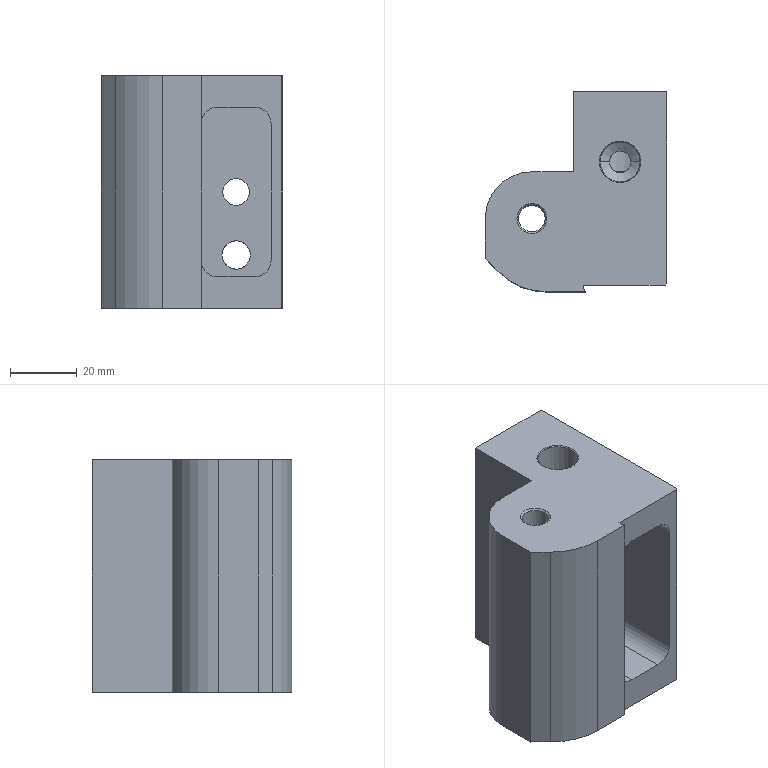Part | STEP file | BCC3 H14_2B | 1 solid | 50 faces | box 54.5 x 60 x 69.8 mm | volume 132555 mm3 | plane 20 | cylinder 18 | cone 12 | commonest cylinder face diameters 8 x4 10 x4 6.5 x2 8.5 x2 12 x2 20 x2